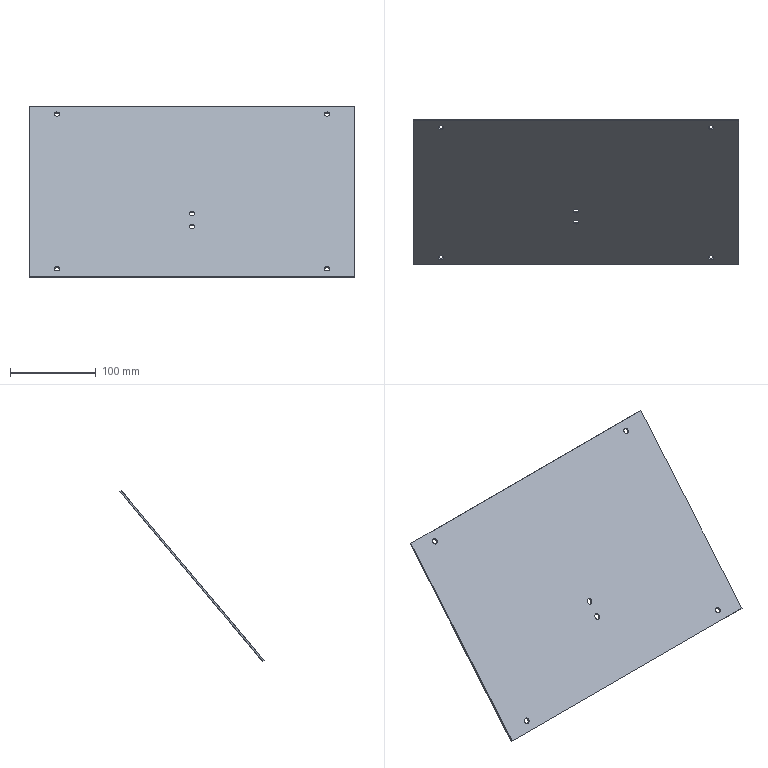Part | SolidWorks | features BaseBody 1 | 1 solid | 18 faces | box 380 x 168.657 x 200.457 mm | volume 197189 mm3 | cylinder 12 | plane 6 | commonest cylinder face diameters 6.5 x8 6.8 x4
STEP:
#1=CARTESIAN_POINT('',(-158.,1.503,-471.241));
#2=VERTEX_POINT('',#1);
#3=CARTESIAN_POINT('',(-158.,-2.675,-476.22));
#4=VERTEX_POINT('',#3);
#5=CARTESIAN_POINT('',(-158.,-0.5861,-473.73));
#6=DIRECTION('',(0.,-0.766,0.6428));
#7=DIRECTION('',(0.,-0.6428,-0.766));
#8=AXIS2_PLACEMENT_3D('',#5,#6,#7);
#9=CIRCLE('',#8,3.25);
#10=EDGE_CURVE('',#2,#4,#9,.T.);
#11=ORIENTED_EDGE('',*,*,#10,.F.);
#12=CARTESIAN_POINT('',(-158.,-0.02909,-469.955));
#13=VERTEX_POINT('',#12);
#14=CARTESIAN_POINT('',(-158.,-0.02909,-469.955));
#15=DIRECTION('',(0.,-0.766,0.6428));
#16=VECTOR('',#15,1000.);
#17=LINE('',#14,#16);
#18=EDGE_CURVE('',#2,#13,#17,.T.);
#19=ORIENTED_EDGE('',*,*,#18,.T.);
#20=CARTESIAN_POINT('',(-158.,-4.207,-474.934));
#21=VERTEX_POINT('',#20);
#22=CARTESIAN_POINT('',(-158.,-2.118,-472.445));
#23=DIRECTION('',(0.,-0.766,0.6428));
#24=DIRECTION('',(0.,-0.6428,-0.766));
#25=AXIS2_PLACEMENT_3D('',#22,#23,#24);
#26=CIRCLE('',#25,3.25);
#27=EDGE_CURVE('',#13,#21,#26,.T.);
#28=ORIENTED_EDGE('',*,*,#27,.T.);
#29=CARTESIAN_POINT('',(-158.,-4.207,-474.934));
#30=DIRECTION('',(0.,-0.766,0.6428));
#31=VECTOR('',#30,1000.);
#32=LINE('',#29,#31);
#33=EDGE_CURVE('',#4,#21,#32,.T.);
#34=ORIENTED_EDGE('',*,*,#33,.F.);
#35=EDGE_LOOP('',(#11,#19,#28,#34));
#36=FACE_OUTER_BOUND('',#35,.T.);
#37=CARTESIAN_POINT('',(-158.,-2.118,-472.445));
#38=DIRECTION('',(0.,-0.766,0.6428));
#39=DIRECTION('',(0.,-0.6428,-0.766));
#40=AXIS2_PLACEMENT_3D('',#37,#38,#39);
#41=CYLINDRICAL_SURFACE('',#40,3.25);
#42=ADVANCED_FACE('',(#36),#41,.F.);
#43=CARTESIAN_POINT('',(-158.,153.201,-290.454));
#44=VERTEX_POINT('',#43);
#45=CARTESIAN_POINT('',(-158.,149.023,-295.433));
#46=VERTEX_POINT('',#45);
#47=CARTESIAN_POINT('',(-158.,151.112,-292.944));
#48=DIRECTION('',(0.,-0.766,0.6428));
#49=DIRECTION('',(0.,-0.6428,-0.766));
#50=AXIS2_PLACEMENT_3D('',#47,#48,#49);
#51=CIRCLE('',#50,3.25);
#52=EDGE_CURVE('',#44,#46,#51,.T.);
#53=ORIENTED_EDGE('',*,*,#52,.F.);
#54=CARTESIAN_POINT('',(-158.,151.669,-289.169));
#55=VERTEX_POINT('',#54);
#56=CARTESIAN_POINT('',(-158.,151.669,-289.169));
#57=DIRECTION('',(0.,-0.766,0.6428));
#58=VECTOR('',#57,1000.);
#59=LINE('',#56,#58);
#60=EDGE_CURVE('',#44,#55,#59,.T.);
#61=ORIENTED_EDGE('',*,*,#60,.T.);
#62=CARTESIAN_POINT('',(-158.,147.491,-294.148));
#63=VERTEX_POINT('',#62);
#64=CARTESIAN_POINT('',(-158.,149.58,-291.658));
#65=DIRECTION('',(0.,-0.766,0.6428));
#66=DIRECTION('',(0.,-0.6428,-0.766));
#67=AXIS2_PLACEMENT_3D('',#64,#65,#66);
#68=CIRCLE('',#67,3.25);
#69=EDGE_CURVE('',#55,#63,#68,.T.);
#70=ORIENTED_EDGE('',*,*,#69,.T.);
#71=CARTESIAN_POINT('',(-158.,147.491,-294.148));
#72=DIRECTION('',(0.,-0.766,0.6428));
#73=VECTOR('',#72,1000.);
#74=LINE('',#71,#73);
#75=EDGE_CURVE('',#46,#63,#74,.T.);
#76=ORIENTED_EDGE('',*,*,#75,.F.);
#77=EDGE_LOOP('',(#53,#61,#70,#76));
#78=FACE_OUTER_BOUND('',#77,.T.);
#79=CARTESIAN_POINT('',(-158.,149.58,-291.658));
#80=DIRECTION('',(0.,-0.766,0.6428));
#81=DIRECTION('',(0.,-0.6428,-0.766));
#82=AXIS2_PLACEMENT_3D('',#79,#80,#81);
#83=CYLINDRICAL_SURFACE('',#82,3.25);
#84=ADVANCED_FACE('',(#78),#83,.F.);
#85=CARTESIAN_POINT('',(158.,153.201,-290.454));
#86=VERTEX_POINT('',#85);
#87=CARTESIAN_POINT('',(158.,149.023,-295.433));
#88=VERTEX_POINT('',#87);
#89=CARTESIAN_POINT('',(158.,151.112,-292.944));
#90=DIRECTION('',(0.,-0.766,0.6428));
#91=DIRECTION('',(0.,-0.6428,-0.766));
#92=AXIS2_PLACEMENT_3D('',#89,#90,#91);
#93=CIRCLE('',#92,3.25);
#94=EDGE_CURVE('',#86,#88,#93,.T.);
#95=ORIENTED_EDGE('',*,*,#94,.F.);
#96=CARTESIAN_POINT('',(158.,151.669,-289.169));
#97=VERTEX_POINT('',#96);
#98=CARTESIAN_POINT('',(158.,151.669,-289.169));
#99=DIRECTION('',(0.,-0.766,0.6428));
#100=VECTOR('',#99,1000.);
#101=LINE('',#98,#100);
#102=EDGE_CURVE('',#86,#97,#101,.T.);
#103=ORIENTED_EDGE('',*,*,#102,.T.);
#104=CARTESIAN_POINT('',(158.,147.491,-294.148));
#105=VERTEX_POINT('',#104);
#106=CARTESIAN_POINT('',(158.,149.58,-291.658));
#107=DIRECTION('',(0.,-0.766,0.6428));
#108=DIRECTION('',(0.,-0.6428,-0.766));
#109=AXIS2_PLACEMENT_3D('',#106,#107,#108);
#110=CIRCLE('',#109,3.25);
#111=EDGE_CURVE('',#97,#105,#110,.T.);
#112=ORIENTED_EDGE('',*,*,#111,.T.);
#113=CARTESIAN_POINT('',(158.,147.491,-294.148));
#114=DIRECTION('',(0.,-0.766,0.6428));
#115=VECTOR('',#114,1000.);
#116=LINE('',#113,#115);
#117=EDGE_CURVE('',#88,#105,#116,.T.);
#118=ORIENTED_EDGE('',*,*,#117,.F.);
#119=EDGE_LOOP('',(#95,#103,#112,#118));
#120=FACE_OUTER_BOUND('',#119,.T.);
#121=CARTESIAN_POINT('',(158.,149.58,-291.658));
#122=DIRECTION('',(0.,-0.766,0.6428));
#123=DIRECTION('',(0.,-0.6428,-0.766));
#124=AXIS2_PLACEMENT_3D('',#121,#122,#123);
#125=CYLINDRICAL_SURFACE('',#124,3.25);
#126=ADVANCED_FACE('',(#120),#125,.F.);
#127=CARTESIAN_POINT('',(158.,1.503,-471.241));
#128=VERTEX_POINT('',#127);
#129=CARTESIAN_POINT('',(158.,-2.675,-476.22));
#130=VERTEX_POINT('',#129);
#131=CARTESIAN_POINT('',(158.,-0.5861,-473.73));
#132=DIRECTION('',(0.,-0.766,0.6428));
#133=DIRECTION('',(0.,-0.6428,-0.766));
#134=AXIS2_PLACEMENT_3D('',#131,#132,#133);
#135=CIRCLE('',#134,3.25);
#136=EDGE_CURVE('',#128,#130,#135,.T.);
#137=ORIENTED_EDGE('',*,*,#136,.F.);
#138=CARTESIAN_POINT('',(158.,-0.02909,-469.955));
#139=VERTEX_POINT('',#138);
#140=CARTESIAN_POINT('',(158.,-0.02909,-469.955));
#141=DIRECTION('',(0.,-0.766,0.6428));
#142=VECTOR('',#141,1000.);
#143=LINE('',#140,#142);
#144=EDGE_CURVE('',#128,#139,#143,.T.);
#145=ORIENTED_EDGE('',*,*,#144,.T.);
#146=CARTESIAN_POINT('',(158.,-4.207,-474.934));
#147=VERTEX_POINT('',#146);
#148=CARTESIAN_POINT('',(158.,-2.118,-472.445));
#149=DIRECTION('',(0.,-0.766,0.6428));
#150=DIRECTION('',(0.,-0.6428,-0.766));
#151=AXIS2_PLACEMENT_3D('',#148,#149,#150);
#152=CIRCLE('',#151,3.25);
#153=EDGE_CURVE('',#139,#147,#152,.T.);
#154=ORIENTED_EDGE('',*,*,#153,.T.);
#155=CARTESIAN_POINT('',(158.,-4.207,-474.934));
#156=DIRECTION('',(0.,-0.766,0.6428));
#157=VECTOR('',#156,1000.);
#158=LINE('',#155,#157);
#159=EDGE_CURVE('',#130,#147,#158,.T.);
#160=ORIENTED_EDGE('',*,*,#159,.F.);
#161=EDGE_LOOP('',(#137,#145,#154,#160));
#162=FACE_OUTER_BOUND('',#161,.T.);
#163=CARTESIAN_POINT('',(158.,-2.118,-472.445));
#164=DIRECTION('',(0.,-0.766,0.6428));
#165=DIRECTION('',(0.,-0.6428,-0.766));
#166=AXIS2_PLACEMENT_3D('',#163,#164,#165);
#167=CYLINDRICAL_SURFACE('',#166,3.25);
#168=ADVANCED_FACE('',(#162),#167,.F.);
#169=CARTESIAN_POINT('',(0.,43.019,-421.763));
#170=VERTEX_POINT('',#169);
#171=CARTESIAN_POINT('',(0.,38.649,-426.972));
#172=VERTEX_POINT('',#171);
#173=CARTESIAN_POINT('',(0.,40.834,-424.368));
#174=DIRECTION('',(0.,-0.766,0.6428));
#175=DIRECTION('',(0.,-0.6428,-0.766));
#176=AXIS2_PLACEMENT_3D('',#173,#174,#175);
#177=CIRCLE('',#176,3.4);
#178=EDGE_CURVE('',#170,#172,#177,.T.);
#179=ORIENTED_EDGE('',*,*,#178,.F.);
#180=CARTESIAN_POINT('',(0.,41.487,-420.478));
#181=VERTEX_POINT('',#180);
#182=CARTESIAN_POINT('',(0.,41.487,-420.478));
#183=DIRECTION('',(0.,-0.766,0.6428));
#184=VECTOR('',#183,1000.);
#185=LINE('',#182,#184);
#186=EDGE_CURVE('',#170,#181,#185,.T.);
#187=ORIENTED_EDGE('',*,*,#186,.T.);
#188=CARTESIAN_POINT('',(0.,37.116,-425.687));
#189=VERTEX_POINT('',#188);
#190=CARTESIAN_POINT('',(0.,39.302,-423.082));
#191=DIRECTION('',(0.,-0.766,0.6428));
#192=DIRECTION('',(0.,-0.6428,-0.766));
#193=AXIS2_PLACEMENT_3D('',#190,#191,#192);
#194=CIRCLE('',#193,3.4);
#195=EDGE_CURVE('',#181,#189,#194,.T.);
#196=ORIENTED_EDGE('',*,*,#195,.T.);
#197=CARTESIAN_POINT('',(0.,37.116,-425.687));
#198=DIRECTION('',(0.,-0.766,0.6428));
#199=VECTOR('',#198,1000.);
#200=LINE('',#197,#199);
#201=EDGE_CURVE('',#172,#189,#200,.T.);
#202=ORIENTED_EDGE('',*,*,#201,.F.);
#203=EDGE_LOOP('',(#179,#187,#196,#202));
#204=FACE_OUTER_BOUND('',#203,.T.);
#205=CARTESIAN_POINT('',(0.,39.302,-423.082));
#206=DIRECTION('',(0.,-0.766,0.6428));
#207=DIRECTION('',(0.,-0.6428,-0.766));
#208=AXIS2_PLACEMENT_3D('',#205,#206,#207);
#209=CYLINDRICAL_SURFACE('',#208,3.4);
#210=ADVANCED_FACE('',(#204),#209,.F.);
#211=CARTESIAN_POINT('',(0.,55.875,-406.442));
#212=VERTEX_POINT('',#211);
#213=CARTESIAN_POINT('',(0.,51.504,-411.651));
#214=VERTEX_POINT('',#213);
#215=CARTESIAN_POINT('',(0.,53.69,-409.047));
#216=DIRECTION('',(0.,-0.766,0.6428));
#217=DIRECTION('',(0.,-0.6428,-0.766));
#218=AXIS2_PLACEMENT_3D('',#215,#216,#217);
#219=CIRCLE('',#218,3.4);
#220=EDGE_CURVE('',#212,#214,#219,.T.);
#221=ORIENTED_EDGE('',*,*,#220,.F.);
#222=CARTESIAN_POINT('',(0.,54.343,-405.157));
#223=VERTEX_POINT('',#222);
#224=CARTESIAN_POINT('',(0.,54.343,-405.157));
#225=DIRECTION('',(0.,-0.766,0.6428));
#226=VECTOR('',#225,1000.);
#227=LINE('',#224,#226);
#228=EDGE_CURVE('',#212,#223,#227,.T.);
#229=ORIENTED_EDGE('',*,*,#228,.T.);
#230=CARTESIAN_POINT('',(0.,49.972,-410.366));
#231=VERTEX_POINT('',#230);
#232=CARTESIAN_POINT('',(0.,52.158,-407.761));
#233=DIRECTION('',(0.,-0.766,0.6428));
#234=DIRECTION('',(0.,-0.6428,-0.766));
#235=AXIS2_PLACEMENT_3D('',#232,#233,#234);
#236=CIRCLE('',#235,3.4);
#237=EDGE_CURVE('',#223,#231,#236,.T.);
#238=ORIENTED_EDGE('',*,*,#237,.T.);
#239=CARTESIAN_POINT('',(0.,49.972,-410.366));
#240=DIRECTION('',(0.,-0.766,0.6428));
#241=VECTOR('',#240,1000.);
#242=LINE('',#239,#241);
#243=EDGE_CURVE('',#214,#231,#242,.T.);
#244=ORIENTED_EDGE('',*,*,#243,.F.);
#245=EDGE_LOOP('',(#221,#229,#238,#244));
#246=FACE_OUTER_BOUND('',#245,.T.);
#247=CARTESIAN_POINT('',(0.,52.158,-407.761));
#248=DIRECTION('',(0.,-0.766,0.6428));
#249=DIRECTION('',(0.,-0.6428,-0.766));
#250=AXIS2_PLACEMENT_3D('',#247,#248,#249);
#251=CYLINDRICAL_SURFACE('',#250,3.4);
#252=ADVANCED_FACE('',(#246),#251,.F.);
#253=CARTESIAN_POINT('',(190.,-9.832,-481.637));
#254=VERTEX_POINT('',#253);
#255=CARTESIAN_POINT('',(-190.,-9.832,-481.637));
#256=VERTEX_POINT('',#255);
#257=CARTESIAN_POINT('',(0.,-9.832,-481.637));
#258=DIRECTION('',(-1.,0.,0.));
#259=VECTOR('',#258,1000.);
#260=LINE('',#257,#259);
#261=EDGE_CURVE('',#254,#256,#260,.T.);
#262=ORIENTED_EDGE('',*,*,#261,.F.);
#263=CARTESIAN_POINT('',(190.,157.293,-282.466));
#264=VERTEX_POINT('',#263);
#265=CARTESIAN_POINT('',(190.,73.731,-382.051));
#266=DIRECTION('',(0.,-0.6428,-0.766));
#267=VECTOR('',#266,1000.);
#268=LINE('',#265,#267);
#269=EDGE_CURVE('',#264,#254,#268,.T.);
#270=ORIENTED_EDGE('',*,*,#269,.F.);
#271=CARTESIAN_POINT('',(-190.,157.293,-282.466));
#272=VERTEX_POINT('',#271);
#273=CARTESIAN_POINT('',(0.,157.293,-282.466));
#274=DIRECTION('',(1.,0.,0.));
#275=VECTOR('',#274,1000.);
#276=LINE('',#273,#275);
#277=EDGE_CURVE('',#272,#264,#276,.T.);
#278=ORIENTED_EDGE('',*,*,#277,.F.);
#279=CARTESIAN_POINT('',(-190.,73.731,-382.051));
#280=DIRECTION('',(0.,0.6428,0.766));
#281=VECTOR('',#280,1000.);
#282=LINE('',#279,#281);
#283=EDGE_CURVE('',#256,#272,#282,.T.);
#284=ORIENTED_EDGE('',*,*,#283,.F.);
#285=EDGE_LOOP('',(#262,#270,#278,#284));
#286=FACE_OUTER_BOUND('',#285,.T.);
#287=CARTESIAN_POINT('',(-158.,-2.118,-472.445));
#288=DIRECTION('',(0.,-0.766,0.6428));
#289=DIRECTION('',(0.,-0.6428,-0.766));
#290=AXIS2_PLACEMENT_3D('',#287,#288,#289);
#291=CIRCLE('',#290,3.25);
#292=EDGE_CURVE('',#21,#13,#291,.T.);
#293=ORIENTED_EDGE('',*,*,#292,.F.);
#294=ORIENTED_EDGE('',*,*,#27,.F.);
#295=EDGE_LOOP('',(#293,#294));
#296=FACE_BOUND('',#295,.T.);
#297=CARTESIAN_POINT('',(-158.,149.58,-291.658));
#298=DIRECTION('',(0.,-0.766,0.6428));
#299=DIRECTION('',(0.,-0.6428,-0.766));
#300=AXIS2_PLACEMENT_3D('',#297,#298,#299);
#301=CIRCLE('',#300,3.25);
#302=EDGE_CURVE('',#63,#55,#301,.T.);
#303=ORIENTED_EDGE('',*,*,#302,.F.);
#304=ORIENTED_EDGE('',*,*,#69,.F.);
#305=EDGE_LOOP('',(#303,#304));
#306=FACE_BOUND('',#305,.T.);
#307=CARTESIAN_POINT('',(158.,149.58,-291.658));
#308=DIRECTION('',(0.,-0.766,0.6428));
#309=DIRECTION('',(0.,-0.6428,-0.766));
#310=AXIS2_PLACEMENT_3D('',#307,#308,#309);
#311=CIRCLE('',#310,3.25);
#312=EDGE_CURVE('',#105,#97,#311,.T.);
#313=ORIENTED_EDGE('',*,*,#312,.F.);
#314=ORIENTED_EDGE('',*,*,#111,.F.);
#315=EDGE_LOOP('',(#313,#314));
#316=FACE_BOUND('',#315,.T.);
#317=CARTESIAN_POINT('',(158.,-2.118,-472.445));
#318=DIRECTION('',(0.,-0.766,0.6428));
#319=DIRECTION('',(0.,-0.6428,-0.766));
#320=AXIS2_PLACEMENT_3D('',#317,#318,#319);
#321=CIRCLE('',#320,3.25);
#322=EDGE_CURVE('',#147,#139,#321,.T.);
#323=ORIENTED_EDGE('',*,*,#322,.F.);
#324=ORIENTED_EDGE('',*,*,#153,.F.);
#325=EDGE_LOOP('',(#323,#324));
#326=FACE_BOUND('',#325,.T.);
#327=CARTESIAN_POINT('',(0.,39.302,-423.082));
#328=DIRECTION('',(0.,-0.766,0.6428));
#329=DIRECTION('',(0.,-0.6428,-0.766));
#330=AXIS2_PLACEMENT_3D('',#327,#328,#329);
#331=CIRCLE('',#330,3.4);
#332=EDGE_CURVE('',#189,#181,#331,.T.);
#333=ORIENTED_EDGE('',*,*,#332,.F.);
#334=ORIENTED_EDGE('',*,*,#195,.F.);
#335=EDGE_LOOP('',(#333,#334));
#336=FACE_BOUND('',#335,.T.);
#337=CARTESIAN_POINT('',(0.,52.158,-407.761));
#338=DIRECTION('',(0.,-0.766,0.6428));
#339=DIRECTION('',(0.,-0.6428,-0.766));
#340=AXIS2_PLACEMENT_3D('',#337,#338,#339);
#341=CIRCLE('',#340,3.4);
#342=EDGE_CURVE('',#231,#223,#341,.T.);
#343=ORIENTED_EDGE('',*,*,#342,.F.);
#344=ORIENTED_EDGE('',*,*,#237,.F.);
#345=EDGE_LOOP('',(#343,#344));
#346=FACE_BOUND('',#345,.T.);
#347=CARTESIAN_POINT('',(0.,73.731,-382.051));
#348=DIRECTION('',(0.,0.766,-0.6428));
#349=DIRECTION('',(0.,0.6428,0.766));
#350=AXIS2_PLACEMENT_3D('',#347,#348,#349);
#351=PLANE('',#350);
#352=ADVANCED_FACE('',(#286,#296,#306,#316,#326,#336,#346),#351,.F.);
#353=CARTESIAN_POINT('',(-190.,158.825,-283.751));
#354=VERTEX_POINT('',#353);
#355=CARTESIAN_POINT('',(-190.,158.825,-283.751));
#356=DIRECTION('',(0.,-0.766,0.6428));
#357=VECTOR('',#356,1000.);
#358=LINE('',#355,#357);
#359=EDGE_CURVE('',#354,#272,#358,.T.);
#360=ORIENTED_EDGE('',*,*,#359,.F.);
#361=CARTESIAN_POINT('',(-190.,-8.3,-482.923));
#362=VERTEX_POINT('',#361);
#363=CARTESIAN_POINT('',(-190.,-8.3,-482.923));
#364=DIRECTION('',(0.,0.6428,0.766));
#365=VECTOR('',#364,1000.);
#366=LINE('',#363,#365);
#367=EDGE_CURVE('',#362,#354,#366,.T.);
#368=ORIENTED_EDGE('',*,*,#367,.F.);
#369=CARTESIAN_POINT('',(-190.,-9.832,-481.637));
#370=DIRECTION('',(0.,0.766,-0.6428));
#371=VECTOR('',#370,1000.);
#372=LINE('',#369,#371);
#373=EDGE_CURVE('',#256,#362,#372,.T.);
#374=ORIENTED_EDGE('',*,*,#373,.F.);
#375=ORIENTED_EDGE('',*,*,#283,.T.);
#376=EDGE_LOOP('',(#360,#368,#374,#375));
#377=FACE_OUTER_BOUND('',#376,.T.);
#378=CARTESIAN_POINT('',(-190.,158.825,-283.751));
#379=DIRECTION('',(1.,0.,0.));
#380=DIRECTION('',(0.,0.,-1.));
#381=AXIS2_PLACEMENT_3D('',#378,#379,#380);
#382=PLANE('',#381);
#383=ADVANCED_FACE('',(#377),#382,.F.);
#384=ORIENTED_EDGE('',*,*,#373,.T.);
#385=CARTESIAN_POINT('',(190.,-8.3,-482.923));
#386=VERTEX_POINT('',#385);
#387=CARTESIAN_POINT('',(190.,-8.3,-482.923));
#388=DIRECTION('',(-1.,0.,0.));
#389=VECTOR('',#388,1000.);
#390=LINE('',#387,#389);
#391=EDGE_CURVE('',#386,#362,#390,.T.);
#392=ORIENTED_EDGE('',*,*,#391,.F.);
#393=CARTESIAN_POINT('',(190.,-8.3,-482.923));
#394=DIRECTION('',(0.,0.766,-0.6428));
#395=VECTOR('',#394,1000.);
#396=LINE('',#393,#395);
#397=EDGE_CURVE('',#254,#386,#396,.T.);
#398=ORIENTED_EDGE('',*,*,#397,.F.);
#399=ORIENTED_EDGE('',*,*,#261,.T.);
#400=EDGE_LOOP('',(#384,#392,#398,#399));
#401=FACE_OUTER_BOUND('',#400,.T.);
#402=CARTESIAN_POINT('',(190.,-8.3,-482.923));
#403=DIRECTION('',(0.,0.6428,0.766));
#404=DIRECTION('',(0.,-0.766,0.6428));
#405=AXIS2_PLACEMENT_3D('',#402,#403,#404);
#406=PLANE('',#405);
#407=ADVANCED_FACE('',(#401),#406,.F.);
#408=ORIENTED_EDGE('',*,*,#397,.T.);
#409=CARTESIAN_POINT('',(190.,158.825,-283.751));
#410=VERTEX_POINT('',#409);
#411=CARTESIAN_POINT('',(190.,158.825,-283.751));
#412=DIRECTION('',(0.,-0.6428,-0.766));
#413=VECTOR('',#412,1000.);
#414=LINE('',#411,#413);
#415=EDGE_CURVE('',#410,#386,#414,.T.);
#416=ORIENTED_EDGE('',*,*,#415,.F.);
#417=CARTESIAN_POINT('',(190.,157.293,-282.466));
#418=DIRECTION('',(0.,0.766,-0.6428));
#419=VECTOR('',#418,1000.);
#420=LINE('',#417,#419);
#421=EDGE_CURVE('',#264,#410,#420,.T.);
#422=ORIENTED_EDGE('',*,*,#421,.F.);
#423=ORIENTED_EDGE('',*,*,#269,.T.);
#424=EDGE_LOOP('',(#408,#416,#422,#423));
#425=FACE_OUTER_BOUND('',#424,.T.);
#426=CARTESIAN_POINT('',(190.,158.825,-283.751));
#427=DIRECTION('',(-1.,0.,0.));
#428=DIRECTION('',(0.,0.,1.));
#429=AXIS2_PLACEMENT_3D('',#426,#427,#428);
#430=PLANE('',#429);
#431=ADVANCED_FACE('',(#425),#430,.F.);
#432=ORIENTED_EDGE('',*,*,#421,.T.);
#433=CARTESIAN_POINT('',(190.,158.825,-283.751));
#434=DIRECTION('',(1.,0.,0.));
#435=VECTOR('',#434,1000.);
#436=LINE('',#433,#435);
#437=EDGE_CURVE('',#354,#410,#436,.T.);
#438=ORIENTED_EDGE('',*,*,#437,.F.);
#439=ORIENTED_EDGE('',*,*,#359,.T.);
#440=ORIENTED_EDGE('',*,*,#277,.T.);
#441=EDGE_LOOP('',(#432,#438,#439,#440));
#442=FACE_OUTER_BOUND('',#441,.T.);
#443=CARTESIAN_POINT('',(190.,158.825,-283.751));
#444=DIRECTION('',(0.,-0.6428,-0.766));
#445=DIRECTION('',(0.,0.766,-0.6428));
#446=AXIS2_PLACEMENT_3D('',#443,#444,#445);
#447=PLANE('',#446);
#448=ADVANCED_FACE('',(#442),#447,.F.);
#449=ORIENTED_EDGE('',*,*,#18,.F.);
#450=CARTESIAN_POINT('',(-158.,-0.5861,-473.73));
#451=DIRECTION('',(0.,-0.766,0.6428));
#452=DIRECTION('',(0.,-0.6428,-0.766));
#453=AXIS2_PLACEMENT_3D('',#450,#451,#452);
#454=CIRCLE('',#453,3.25);
#455=EDGE_CURVE('',#4,#2,#454,.T.);
#456=ORIENTED_EDGE('',*,*,#455,.F.);
#457=ORIENTED_EDGE('',*,*,#33,.T.);
#458=ORIENTED_EDGE('',*,*,#292,.T.);
#459=EDGE_LOOP('',(#449,#456,#457,#458));
#460=FACE_OUTER_BOUND('',#459,.T.);
#461=CARTESIAN_POINT('',(-158.,-2.118,-472.445));
#462=DIRECTION('',(0.,-0.766,0.6428));
#463=DIRECTION('',(0.,-0.6428,-0.766));
#464=AXIS2_PLACEMENT_3D('',#461,#462,#463);
#465=CYLINDRICAL_SURFACE('',#464,3.25);
#466=ADVANCED_FACE('',(#460),#465,.F.);
#467=ORIENTED_EDGE('',*,*,#60,.F.);
#468=CARTESIAN_POINT('',(-158.,151.112,-292.944));
#469=DIRECTION('',(0.,-0.766,0.6428));
#470=DIRECTION('',(0.,-0.6428,-0.766));
#471=AXIS2_PLACEMENT_3D('',#468,#469,#470);
#472=CIRCLE('',#471,3.25);
#473=EDGE_CURVE('',#46,#44,#472,.T.);
#474=ORIENTED_EDGE('',*,*,#473,.F.);
#475=ORIENTED_EDGE('',*,*,#75,.T.);
#476=ORIENTED_EDGE('',*,*,#302,.T.);
#477=EDGE_LOOP('',(#467,#474,#475,#476));
#478=FACE_OUTER_BOUND('',#477,.T.);
#479=CARTESIAN_POINT('',(-158.,149.58,-291.658));
#480=DIRECTION('',(0.,-0.766,0.6428));
#481=DIRECTION('',(0.,-0.6428,-0.766));
#482=AXIS2_PLACEMENT_3D('',#479,#480,#481);
#483=CYLINDRICAL_SURFACE('',#482,3.25);
#484=ADVANCED_FACE('',(#478),#483,.F.);
#485=ORIENTED_EDGE('',*,*,#102,.F.);
#486=CARTESIAN_POINT('',(158.,151.112,-292.944));
#487=DIRECTION('',(0.,-0.766,0.6428));
#488=DIRECTION('',(0.,-0.6428,-0.766));
#489=AXIS2_PLACEMENT_3D('',#486,#487,#488);
#490=CIRCLE('',#489,3.25);
#491=EDGE_CURVE('',#88,#86,#490,.T.);
#492=ORIENTED_EDGE('',*,*,#491,.F.);
#493=ORIENTED_EDGE('',*,*,#117,.T.);
#494=ORIENTED_EDGE('',*,*,#312,.T.);
#495=EDGE_LOOP('',(#485,#492,#493,#494));
#496=FACE_OUTER_BOUND('',#495,.T.);
#497=CARTESIAN_POINT('',(158.,149.58,-291.658));
#498=DIRECTION('',(0.,-0.766,0.6428));
#499=DIRECTION('',(0.,-0.6428,-0.766));
#500=AXIS2_PLACEMENT_3D('',#497,#498,#499);
#501=CYLINDRICAL_SURFACE('',#500,3.25);
#502=ADVANCED_FACE('',(#496),#501,.F.);
#503=ORIENTED_EDGE('',*,*,#144,.F.);
#504=CARTESIAN_POINT('',(158.,-0.5861,-473.73));
#505=DIRECTION('',(0.,-0.766,0.6428));
#506=DIRECTION('',(0.,-0.6428,-0.766));
#507=AXIS2_PLACEMENT_3D('',#504,#505,#506);
#508=CIRCLE('',#507,3.25);
#509=EDGE_CURVE('',#130,#128,#508,.T.);
#510=ORIENTED_EDGE('',*,*,#509,.F.);
#511=ORIENTED_EDGE('',*,*,#159,.T.);
#512=ORIENTED_EDGE('',*,*,#322,.T.);
#513=EDGE_LOOP('',(#503,#510,#511,#512));
#514=FACE_OUTER_BOUND('',#513,.T.);
#515=CARTESIAN_POINT('',(158.,-2.118,-472.445));
#516=DIRECTION('',(0.,-0.766,0.6428));
#517=DIRECTION('',(0.,-0.6428,-0.766));
#518=AXIS2_PLACEMENT_3D('',#515,#516,#517);
#519=CYLINDRICAL_SURFACE('',#518,3.25);
#520=ADVANCED_FACE('',(#514),#519,.F.);
#521=ORIENTED_EDGE('',*,*,#186,.F.);
#522=CARTESIAN_POINT('',(0.,40.834,-424.368));
#523=DIRECTION('',(0.,-0.766,0.6428));
#524=DIRECTION('',(0.,-0.6428,-0.766));
#525=AXIS2_PLACEMENT_3D('',#522,#523,#524);
#526=CIRCLE('',#525,3.4);
#527=EDGE_CURVE('',#172,#170,#526,.T.);
#528=ORIENTED_EDGE('',*,*,#527,.F.);
#529=ORIENTED_EDGE('',*,*,#201,.T.);
#530=ORIENTED_EDGE('',*,*,#332,.T.);
#531=EDGE_LOOP('',(#521,#528,#529,#530));
#532=FACE_OUTER_BOUND('',#531,.T.);
#533=CARTESIAN_POINT('',(0.,39.302,-423.082));
#534=DIRECTION('',(0.,-0.766,0.6428));
#535=DIRECTION('',(0.,-0.6428,-0.766));
#536=AXIS2_PLACEMENT_3D('',#533,#534,#535);
#537=CYLINDRICAL_SURFACE('',#536,3.4);
#538=ADVANCED_FACE('',(#532),#537,.F.);
#539=ORIENTED_EDGE('',*,*,#228,.F.);
#540=CARTESIAN_POINT('',(0.,53.69,-409.047));
#541=DIRECTION('',(0.,-0.766,0.6428));
#542=DIRECTION('',(0.,-0.6428,-0.766));
#543=AXIS2_PLACEMENT_3D('',#540,#541,#542);
#544=CIRCLE('',#543,3.4);
#545=EDGE_CURVE('',#214,#212,#544,.T.);
#546=ORIENTED_EDGE('',*,*,#545,.F.);
#547=ORIENTED_EDGE('',*,*,#243,.T.);
#548=ORIENTED_EDGE('',*,*,#342,.T.);
#549=EDGE_LOOP('',(#539,#546,#547,#548));
#550=FACE_OUTER_BOUND('',#549,.T.);
#551=CARTESIAN_POINT('',(0.,52.158,-407.761));
#552=DIRECTION('',(0.,-0.766,0.6428));
#553=DIRECTION('',(0.,-0.6428,-0.766));
#554=AXIS2_PLACEMENT_3D('',#551,#552,#553);
#555=CYLINDRICAL_SURFACE('',#554,3.4);
#556=ADVANCED_FACE('',(#550),#555,.F.);
#557=ORIENTED_EDGE('',*,*,#415,.T.);
#558=ORIENTED_EDGE('',*,*,#391,.T.);
#559=ORIENTED_EDGE('',*,*,#367,.T.);
#560=ORIENTED_EDGE('',*,*,#437,.T.);
#561=EDGE_LOOP('',(#557,#558,#559,#560));
#562=FACE_OUTER_BOUND('',#561,.T.);
#563=ORIENTED_EDGE('',*,*,#455,.T.);
#564=ORIENTED_EDGE('',*,*,#10,.T.);
#565=EDGE_LOOP('',(#563,#564));
#566=FACE_BOUND('',#565,.T.);
#567=ORIENTED_EDGE('',*,*,#473,.T.);
#568=ORIENTED_EDGE('',*,*,#52,.T.);
#569=EDGE_LOOP('',(#567,#568));
#570=FACE_BOUND('',#569,.T.);
#571=ORIENTED_EDGE('',*,*,#491,.T.);
#572=ORIENTED_EDGE('',*,*,#94,.T.);
#573=EDGE_LOOP('',(#571,#572));
#574=FACE_BOUND('',#573,.T.);
#575=ORIENTED_EDGE('',*,*,#509,.T.);
#576=ORIENTED_EDGE('',*,*,#136,.T.);
#577=EDGE_LOOP('',(#575,#576));
#578=FACE_BOUND('',#577,.T.);
#579=ORIENTED_EDGE('',*,*,#527,.T.);
#580=ORIENTED_EDGE('',*,*,#178,.T.);
#581=EDGE_LOOP('',(#579,#580));
#582=FACE_BOUND('',#581,.T.);
#583=ORIENTED_EDGE('',*,*,#545,.T.);
#584=ORIENTED_EDGE('',*,*,#220,.T.);
#585=EDGE_LOOP('',(#583,#584));
#586=FACE_BOUND('',#585,.T.);
#587=CARTESIAN_POINT('',(0.,75.263,-383.337));
#588=DIRECTION('',(0.,0.766,-0.6428));
#589=DIRECTION('',(0.,0.6428,0.766));
#590=AXIS2_PLACEMENT_3D('',#587,#588,#589);
#591=PLANE('',#590);
#592=ADVANCED_FACE('',(#562,#566,#570,#574,#578,#582,#586),#591,.T.);
#593=CLOSED_SHELL('',(#42,#84,#126,#168,#210,#252,#352,#383,#407,#431,#448,#466,#484,#502,#520,#538,#556,#592));
#594=MANIFOLD_SOLID_BREP('',#593);
#595=CARTESIAN_POINT('',(0.,0.,0.));
#596=DIRECTION('',(0.,0.,1.));
#597=DIRECTION('',(1.,0.,0.));
#598=AXIS2_PLACEMENT_3D('',#595,#596,#597);
#599=(LENGTH_UNIT()NAMED_UNIT(*)SI_UNIT(.MILLI.,.METRE.));
#600=UNCERTAINTY_MEASURE_WITH_UNIT(LENGTH_MEASURE(0.00001),#599,'','');
#601=(NAMED_UNIT(*)PLANE_ANGLE_UNIT()SI_UNIT($,.RADIAN.));
#602=(NAMED_UNIT(*)SI_UNIT($,.STERADIAN.)SOLID_ANGLE_UNIT());
#603=(GEOMETRIC_REPRESENTATION_CONTEXT(3)GLOBAL_UNCERTAINTY_ASSIGNED_CONTEXT((#600))GLOBAL_UNIT_ASSIGNED_CONTEXT((#599,#601,#602))REPRESENTATION_CONTEXT('',''));
#604=ADVANCED_BREP_SHAPE_REPRESENTATION('',(#594,#598),#603);